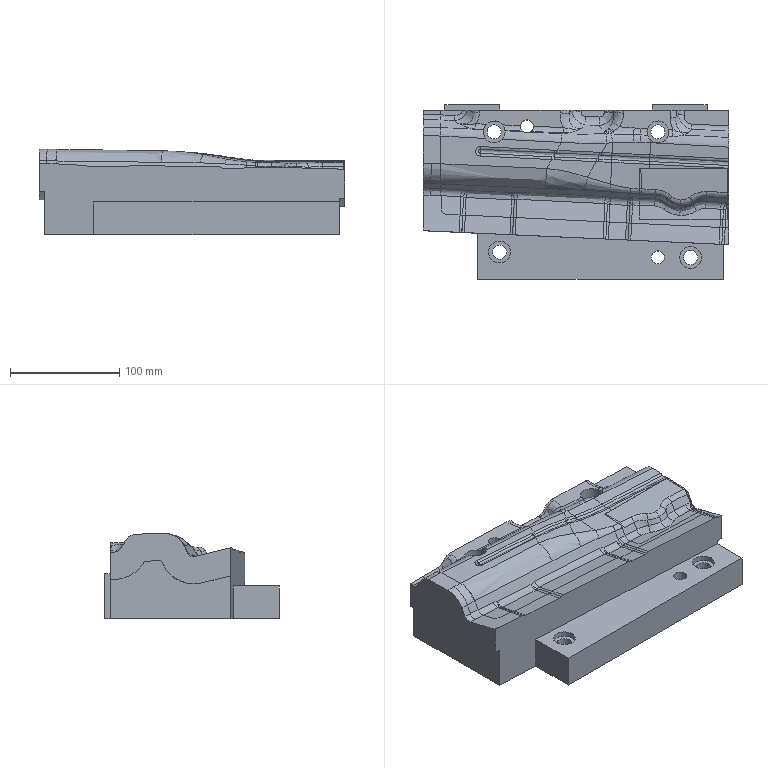Part | NX | features solid 2 | 1 solid | 242 faces | box 280 x 160 x 78.285 mm | volume 2308579 mm3 | spline 205 | plane 27 | cylinder 10 | commonest cylinder face diameters 13 x4 20 x4 12 x2